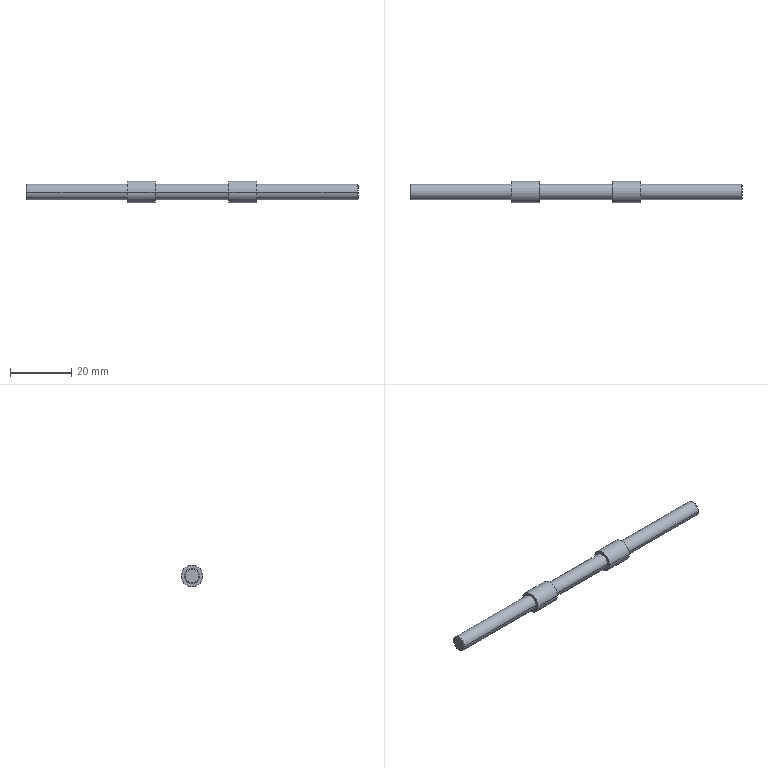Part | SolidWorks | features BaseBody 1 | 1 solid | 20 faces | box 108 x 7 x 7 mm | volume 2459 mm3 | cylinder 10 | plane 6 | cone 4 | commonest cylinder face diameters 5 x6 7 x4
STEP:
#1=CARTESIAN_POINT('',(0.,-2.25,0.));
#2=VERTEX_POINT('',#1);
#3=CARTESIAN_POINT('',(0.,2.25,0.));
#4=VERTEX_POINT('',#3);
#5=CARTESIAN_POINT('',(0.,0.,0.));
#6=DIRECTION('',(1.,0.,0.));
#7=DIRECTION('',(0.,-1.,0.));
#8=AXIS2_PLACEMENT_3D('',#5,#6,#7);
#9=CIRCLE('',#8,2.25);
#10=EDGE_CURVE('',#2,#4,#9,.T.);
#11=ORIENTED_EDGE('',*,*,#10,.T.);
#12=CARTESIAN_POINT('',(0.25,2.5,0.));
#13=VERTEX_POINT('',#12);
#14=CARTESIAN_POINT('',(0.125,2.375,0.));
#15=DIRECTION('',(0.7071,0.7071,0.));
#16=VECTOR('',#15,1000.);
#17=LINE('',#14,#16);
#18=EDGE_CURVE('',#4,#13,#17,.T.);
#19=ORIENTED_EDGE('',*,*,#18,.T.);
#20=CARTESIAN_POINT('',(0.25,-2.5,0.));
#21=VERTEX_POINT('',#20);
#22=CARTESIAN_POINT('',(0.25,0.,0.));
#23=DIRECTION('',(-1.,0.,0.));
#24=DIRECTION('',(0.,-1.,0.));
#25=AXIS2_PLACEMENT_3D('',#22,#23,#24);
#26=CIRCLE('',#25,2.5);
#27=EDGE_CURVE('',#13,#21,#26,.T.);
#28=ORIENTED_EDGE('',*,*,#27,.T.);
#29=CARTESIAN_POINT('',(0.125,-2.375,0.));
#30=DIRECTION('',(0.7071,-0.7071,0.));
#31=VECTOR('',#30,1000.);
#32=LINE('',#29,#31);
#33=EDGE_CURVE('',#2,#21,#32,.T.);
#34=ORIENTED_EDGE('',*,*,#33,.F.);
#35=EDGE_LOOP('',(#11,#19,#28,#34));
#36=FACE_OUTER_BOUND('',#35,.T.);
#37=CARTESIAN_POINT('',(0.125,0.,0.));
#38=DIRECTION('',(1.,0.,0.));
#39=DIRECTION('',(0.,-1.,0.));
#40=AXIS2_PLACEMENT_3D('',#37,#38,#39);
#41=CONICAL_SURFACE('',#40,2.375,0.7854);
#42=ADVANCED_FACE('',(#36),#41,.T.);
#43=CARTESIAN_POINT('',(33.,-2.5,0.));
#44=VERTEX_POINT('',#43);
#45=CARTESIAN_POINT('',(33.,2.5,0.));
#46=VERTEX_POINT('',#45);
#47=CARTESIAN_POINT('',(33.,0.,0.));
#48=DIRECTION('',(1.,0.,0.));
#49=DIRECTION('',(0.,0.,-1.));
#50=AXIS2_PLACEMENT_3D('',#47,#48,#49);
#51=CIRCLE('',#50,2.5);
#52=EDGE_CURVE('',#44,#46,#51,.T.);
#53=ORIENTED_EDGE('',*,*,#52,.F.);
#54=CARTESIAN_POINT('',(19.,-2.5,0.));
#55=DIRECTION('',(-1.,0.,0.));
#56=VECTOR('',#55,1000.);
#57=LINE('',#54,#56);
#58=EDGE_CURVE('',#44,#21,#57,.T.);
#59=ORIENTED_EDGE('',*,*,#58,.T.);
#60=ORIENTED_EDGE('',*,*,#27,.F.);
#61=CARTESIAN_POINT('',(19.,2.5,0.));
#62=DIRECTION('',(-1.,0.,0.));
#63=VECTOR('',#62,1000.);
#64=LINE('',#61,#63);
#65=EDGE_CURVE('',#46,#13,#64,.T.);
#66=ORIENTED_EDGE('',*,*,#65,.F.);
#67=EDGE_LOOP('',(#53,#59,#60,#66));
#68=FACE_OUTER_BOUND('',#67,.T.);
#69=CARTESIAN_POINT('',(19.,0.,0.));
#70=DIRECTION('',(-1.,0.,0.));
#71=DIRECTION('',(0.,1.,0.));
#72=AXIS2_PLACEMENT_3D('',#69,#70,#71);
#73=CYLINDRICAL_SURFACE('',#72,2.5);
#74=ADVANCED_FACE('',(#68),#73,.T.);
#75=CARTESIAN_POINT('',(108.,-2.25,0.));
#76=VERTEX_POINT('',#75);
#77=CARTESIAN_POINT('',(108.,2.25,0.));
#78=VERTEX_POINT('',#77);
#79=CARTESIAN_POINT('',(108.,0.,0.));
#80=DIRECTION('',(-1.,0.,0.));
#81=DIRECTION('',(0.,-1.,0.));
#82=AXIS2_PLACEMENT_3D('',#79,#80,#81);
#83=CIRCLE('',#82,2.25);
#84=EDGE_CURVE('',#76,#78,#83,.T.);
#85=ORIENTED_EDGE('',*,*,#84,.T.);
#86=CARTESIAN_POINT('',(107.75,2.5,0.));
#87=VERTEX_POINT('',#86);
#88=CARTESIAN_POINT('',(107.875,2.375,0.));
#89=DIRECTION('',(-0.7071,0.7071,0.));
#90=VECTOR('',#89,1000.);
#91=LINE('',#88,#90);
#92=EDGE_CURVE('',#78,#87,#91,.T.);
#93=ORIENTED_EDGE('',*,*,#92,.T.);
#94=CARTESIAN_POINT('',(107.75,-2.5,0.));
#95=VERTEX_POINT('',#94);
#96=CARTESIAN_POINT('',(107.75,0.,0.));
#97=DIRECTION('',(1.,0.,0.));
#98=DIRECTION('',(0.,-1.,0.));
#99=AXIS2_PLACEMENT_3D('',#96,#97,#98);
#100=CIRCLE('',#99,2.5);
#101=EDGE_CURVE('',#87,#95,#100,.T.);
#102=ORIENTED_EDGE('',*,*,#101,.T.);
#103=CARTESIAN_POINT('',(107.875,-2.375,0.));
#104=DIRECTION('',(-0.7071,-0.7071,0.));
#105=VECTOR('',#104,1000.);
#106=LINE('',#103,#105);
#107=EDGE_CURVE('',#76,#95,#106,.T.);
#108=ORIENTED_EDGE('',*,*,#107,.F.);
#109=EDGE_LOOP('',(#85,#93,#102,#108));
#110=FACE_OUTER_BOUND('',#109,.T.);
#111=CARTESIAN_POINT('',(107.875,0.,0.));
#112=DIRECTION('',(-1.,0.,0.));
#113=DIRECTION('',(0.,-1.,0.));
#114=AXIS2_PLACEMENT_3D('',#111,#112,#113);
#115=CONICAL_SURFACE('',#114,2.375,0.7854);
#116=ADVANCED_FACE('',(#110),#115,.T.);
#117=CARTESIAN_POINT('',(107.75,0.,0.));
#118=DIRECTION('',(1.,0.,0.));
#119=DIRECTION('',(0.,-1.,0.));
#120=AXIS2_PLACEMENT_3D('',#117,#118,#119);
#121=CIRCLE('',#120,2.5);
#122=EDGE_CURVE('',#95,#87,#121,.T.);
#123=ORIENTED_EDGE('',*,*,#122,.F.);
#124=CARTESIAN_POINT('',(75.,-2.5,0.));
#125=VERTEX_POINT('',#124);
#126=CARTESIAN_POINT('',(91.5,-2.5,0.));
#127=DIRECTION('',(-1.,0.,0.));
#128=VECTOR('',#127,1000.);
#129=LINE('',#126,#128);
#130=EDGE_CURVE('',#95,#125,#129,.T.);
#131=ORIENTED_EDGE('',*,*,#130,.T.);
#132=CARTESIAN_POINT('',(75.,2.5,0.));
#133=VERTEX_POINT('',#132);
#134=CARTESIAN_POINT('',(75.,0.,0.));
#135=DIRECTION('',(1.,0.,0.));
#136=DIRECTION('',(0.,0.,-1.));
#137=AXIS2_PLACEMENT_3D('',#134,#135,#136);
#138=CIRCLE('',#137,2.5);
#139=EDGE_CURVE('',#125,#133,#138,.T.);
#140=ORIENTED_EDGE('',*,*,#139,.T.);
#141=CARTESIAN_POINT('',(91.5,2.5,0.));
#142=DIRECTION('',(-1.,0.,0.));
#143=VECTOR('',#142,1000.);
#144=LINE('',#141,#143);
#145=EDGE_CURVE('',#87,#133,#144,.T.);
#146=ORIENTED_EDGE('',*,*,#145,.F.);
#147=EDGE_LOOP('',(#123,#131,#140,#146));
#148=FACE_OUTER_BOUND('',#147,.T.);
#149=CARTESIAN_POINT('',(91.5,0.,0.));
#150=DIRECTION('',(-1.,0.,0.));
#151=DIRECTION('',(0.,1.,0.));
#152=AXIS2_PLACEMENT_3D('',#149,#150,#151);
#153=CYLINDRICAL_SURFACE('',#152,2.5);
#154=ADVANCED_FACE('',(#148),#153,.T.);
#155=CARTESIAN_POINT('',(42.,-3.5,0.));
#156=VERTEX_POINT('',#155);
#157=CARTESIAN_POINT('',(42.,3.5,0.));
#158=VERTEX_POINT('',#157);
#159=CARTESIAN_POINT('',(42.,0.,0.));
#160=DIRECTION('',(1.,0.,0.));
#161=DIRECTION('',(0.,0.,-1.));
#162=AXIS2_PLACEMENT_3D('',#159,#160,#161);
#163=CIRCLE('',#162,3.5);
#164=EDGE_CURVE('',#156,#158,#163,.T.);
#165=ORIENTED_EDGE('',*,*,#164,.F.);
#166=CARTESIAN_POINT('',(33.,-3.5,0.));
#167=VERTEX_POINT('',#166);
#168=CARTESIAN_POINT('',(37.5,-3.5,0.));
#169=DIRECTION('',(-1.,0.,0.));
#170=VECTOR('',#169,1000.);
#171=LINE('',#168,#170);
#172=EDGE_CURVE('',#156,#167,#171,.T.);
#173=ORIENTED_EDGE('',*,*,#172,.T.);
#174=CARTESIAN_POINT('',(33.,3.5,0.));
#175=VERTEX_POINT('',#174);
#176=CARTESIAN_POINT('',(33.,0.,0.));
#177=DIRECTION('',(1.,0.,0.));
#178=DIRECTION('',(0.,0.,-1.));
#179=AXIS2_PLACEMENT_3D('',#176,#177,#178);
#180=CIRCLE('',#179,3.5);
#181=EDGE_CURVE('',#167,#175,#180,.T.);
#182=ORIENTED_EDGE('',*,*,#181,.T.);
#183=CARTESIAN_POINT('',(37.5,3.5,0.));
#184=DIRECTION('',(-1.,0.,0.));
#185=VECTOR('',#184,1000.);
#186=LINE('',#183,#185);
#187=EDGE_CURVE('',#158,#175,#186,.T.);
#188=ORIENTED_EDGE('',*,*,#187,.F.);
#189=EDGE_LOOP('',(#165,#173,#182,#188));
#190=FACE_OUTER_BOUND('',#189,.T.);
#191=CARTESIAN_POINT('',(37.5,0.,0.));
#192=DIRECTION('',(-1.,0.,0.));
#193=DIRECTION('',(0.,1.,0.));
#194=AXIS2_PLACEMENT_3D('',#191,#192,#193);
#195=CYLINDRICAL_SURFACE('',#194,3.5);
#196=ADVANCED_FACE('',(#190),#195,.T.);
#197=CARTESIAN_POINT('',(66.,-2.5,0.));
#198=VERTEX_POINT('',#197);
#199=CARTESIAN_POINT('',(66.,2.5,0.));
#200=VERTEX_POINT('',#199);
#201=CARTESIAN_POINT('',(66.,0.,0.));
#202=DIRECTION('',(1.,0.,0.));
#203=DIRECTION('',(0.,0.,-1.));
#204=AXIS2_PLACEMENT_3D('',#201,#202,#203);
#205=CIRCLE('',#204,2.5);
#206=EDGE_CURVE('',#198,#200,#205,.T.);
#207=ORIENTED_EDGE('',*,*,#206,.F.);
#208=CARTESIAN_POINT('',(42.,-2.5,0.));
#209=VERTEX_POINT('',#208);
#210=CARTESIAN_POINT('',(54.,-2.5,0.));
#211=DIRECTION('',(-1.,0.,0.));
#212=VECTOR('',#211,1000.);
#213=LINE('',#210,#212);
#214=EDGE_CURVE('',#198,#209,#213,.T.);
#215=ORIENTED_EDGE('',*,*,#214,.T.);
#216=CARTESIAN_POINT('',(42.,2.5,0.));
#217=VERTEX_POINT('',#216);
#218=CARTESIAN_POINT('',(42.,0.,0.));
#219=DIRECTION('',(1.,0.,0.));
#220=DIRECTION('',(0.,0.,-1.));
#221=AXIS2_PLACEMENT_3D('',#218,#219,#220);
#222=CIRCLE('',#221,2.5);
#223=EDGE_CURVE('',#209,#217,#222,.T.);
#224=ORIENTED_EDGE('',*,*,#223,.T.);
#225=CARTESIAN_POINT('',(54.,2.5,0.));
#226=DIRECTION('',(-1.,0.,0.));
#227=VECTOR('',#226,1000.);
#228=LINE('',#225,#227);
#229=EDGE_CURVE('',#200,#217,#228,.T.);
#230=ORIENTED_EDGE('',*,*,#229,.F.);
#231=EDGE_LOOP('',(#207,#215,#224,#230));
#232=FACE_OUTER_BOUND('',#231,.T.);
#233=CARTESIAN_POINT('',(54.,0.,0.));
#234=DIRECTION('',(-1.,0.,0.));
#235=DIRECTION('',(0.,1.,0.));
#236=AXIS2_PLACEMENT_3D('',#233,#234,#235);
#237=CYLINDRICAL_SURFACE('',#236,2.5);
#238=ADVANCED_FACE('',(#232),#237,.T.);
#239=CARTESIAN_POINT('',(75.,-3.5,0.));
#240=VERTEX_POINT('',#239);
#241=CARTESIAN_POINT('',(75.,3.5,0.));
#242=VERTEX_POINT('',#241);
#243=CARTESIAN_POINT('',(75.,0.,0.));
#244=DIRECTION('',(1.,0.,0.));
#245=DIRECTION('',(0.,0.,-1.));
#246=AXIS2_PLACEMENT_3D('',#243,#244,#245);
#247=CIRCLE('',#246,3.5);
#248=EDGE_CURVE('',#240,#242,#247,.T.);
#249=ORIENTED_EDGE('',*,*,#248,.F.);
#250=CARTESIAN_POINT('',(66.,-3.5,0.));
#251=VERTEX_POINT('',#250);
#252=CARTESIAN_POINT('',(70.5,-3.5,0.));
#253=DIRECTION('',(-1.,0.,0.));
#254=VECTOR('',#253,1000.);
#255=LINE('',#252,#254);
#256=EDGE_CURVE('',#240,#251,#255,.T.);
#257=ORIENTED_EDGE('',*,*,#256,.T.);
#258=CARTESIAN_POINT('',(66.,3.5,0.));
#259=VERTEX_POINT('',#258);
#260=CARTESIAN_POINT('',(66.,0.,0.));
#261=DIRECTION('',(1.,0.,0.));
#262=DIRECTION('',(0.,0.,-1.));
#263=AXIS2_PLACEMENT_3D('',#260,#261,#262);
#264=CIRCLE('',#263,3.5);
#265=EDGE_CURVE('',#251,#259,#264,.T.);
#266=ORIENTED_EDGE('',*,*,#265,.T.);
#267=CARTESIAN_POINT('',(70.5,3.5,0.));
#268=DIRECTION('',(-1.,0.,0.));
#269=VECTOR('',#268,1000.);
#270=LINE('',#267,#269);
#271=EDGE_CURVE('',#242,#259,#270,.T.);
#272=ORIENTED_EDGE('',*,*,#271,.F.);
#273=EDGE_LOOP('',(#249,#257,#266,#272));
#274=FACE_OUTER_BOUND('',#273,.T.);
#275=CARTESIAN_POINT('',(70.5,0.,0.));
#276=DIRECTION('',(-1.,0.,0.));
#277=DIRECTION('',(0.,1.,0.));
#278=AXIS2_PLACEMENT_3D('',#275,#276,#277);
#279=CYLINDRICAL_SURFACE('',#278,3.5);
#280=ADVANCED_FACE('',(#274),#279,.T.);
#281=ORIENTED_EDGE('',*,*,#10,.F.);
#282=CARTESIAN_POINT('',(0.,0.,0.));
#283=DIRECTION('',(1.,0.,0.));
#284=DIRECTION('',(0.,-1.,0.));
#285=AXIS2_PLACEMENT_3D('',#282,#283,#284);
#286=CIRCLE('',#285,2.25);
#287=EDGE_CURVE('',#4,#2,#286,.T.);
#288=ORIENTED_EDGE('',*,*,#287,.F.);
#289=EDGE_LOOP('',(#281,#288));
#290=FACE_OUTER_BOUND('',#289,.T.);
#291=CARTESIAN_POINT('',(0.,2.5,0.));
#292=DIRECTION('',(-1.,0.,0.));
#293=DIRECTION('',(0.,0.,1.));
#294=AXIS2_PLACEMENT_3D('',#291,#292,#293);
#295=PLANE('',#294);
#296=ADVANCED_FACE('',(#290),#295,.T.);
#297=ORIENTED_EDGE('',*,*,#84,.F.);
#298=CARTESIAN_POINT('',(108.,0.,0.));
#299=DIRECTION('',(-1.,0.,0.));
#300=DIRECTION('',(0.,-1.,0.));
#301=AXIS2_PLACEMENT_3D('',#298,#299,#300);
#302=CIRCLE('',#301,2.25);
#303=EDGE_CURVE('',#78,#76,#302,.T.);
#304=ORIENTED_EDGE('',*,*,#303,.F.);
#305=EDGE_LOOP('',(#297,#304));
#306=FACE_OUTER_BOUND('',#305,.T.);
#307=CARTESIAN_POINT('',(108.,0.,0.));
#308=DIRECTION('',(1.,0.,0.));
#309=DIRECTION('',(0.,1.,0.));
#310=AXIS2_PLACEMENT_3D('',#307,#308,#309);
#311=PLANE('',#310);
#312=ADVANCED_FACE('',(#306),#311,.T.);
#313=CARTESIAN_POINT('',(33.,0.,0.));
#314=DIRECTION('',(1.,0.,0.));
#315=DIRECTION('',(0.,0.,-1.));
#316=AXIS2_PLACEMENT_3D('',#313,#314,#315);
#317=CIRCLE('',#316,2.5);
#318=EDGE_CURVE('',#46,#44,#317,.T.);
#319=ORIENTED_EDGE('',*,*,#318,.T.);
#320=ORIENTED_EDGE('',*,*,#52,.T.);
#321=EDGE_LOOP('',(#319,#320));
#322=FACE_BOUND('',#321,.T.);
#323=CARTESIAN_POINT('',(33.,0.,0.));
#324=DIRECTION('',(1.,0.,0.));
#325=DIRECTION('',(0.,0.,-1.));
#326=AXIS2_PLACEMENT_3D('',#323,#324,#325);
#327=CIRCLE('',#326,3.5);
#328=EDGE_CURVE('',#175,#167,#327,.T.);
#329=ORIENTED_EDGE('',*,*,#328,.F.);
#330=ORIENTED_EDGE('',*,*,#181,.F.);
#331=EDGE_LOOP('',(#329,#330));
#332=FACE_OUTER_BOUND('',#331,.T.);
#333=CARTESIAN_POINT('',(33.,3.5,0.));
#334=DIRECTION('',(-1.,0.,0.));
#335=DIRECTION('',(0.,0.,1.));
#336=AXIS2_PLACEMENT_3D('',#333,#334,#335);
#337=PLANE('',#336);
#338=ADVANCED_FACE('',(#322,#332),#337,.T.);
#339=CARTESIAN_POINT('',(42.,0.,0.));
#340=DIRECTION('',(1.,0.,0.));
#341=DIRECTION('',(0.,0.,-1.));
#342=AXIS2_PLACEMENT_3D('',#339,#340,#341);
#343=CIRCLE('',#342,2.5);
#344=EDGE_CURVE('',#217,#209,#343,.T.);
#345=ORIENTED_EDGE('',*,*,#344,.F.);
#346=ORIENTED_EDGE('',*,*,#223,.F.);
#347=EDGE_LOOP('',(#345,#346));
#348=FACE_BOUND('',#347,.T.);
#349=CARTESIAN_POINT('',(42.,0.,0.));
#350=DIRECTION('',(1.,0.,0.));
#351=DIRECTION('',(0.,0.,-1.));
#352=AXIS2_PLACEMENT_3D('',#349,#350,#351);
#353=CIRCLE('',#352,3.5);
#354=EDGE_CURVE('',#158,#156,#353,.T.);
#355=ORIENTED_EDGE('',*,*,#354,.T.);
#356=ORIENTED_EDGE('',*,*,#164,.T.);
#357=EDGE_LOOP('',(#355,#356));
#358=FACE_OUTER_BOUND('',#357,.T.);
#359=CARTESIAN_POINT('',(42.,2.5,0.));
#360=DIRECTION('',(1.,0.,0.));
#361=DIRECTION('',(0.,1.,0.));
#362=AXIS2_PLACEMENT_3D('',#359,#360,#361);
#363=PLANE('',#362);
#364=ADVANCED_FACE('',(#348,#358),#363,.T.);
#365=CARTESIAN_POINT('',(66.,0.,0.));
#366=DIRECTION('',(1.,0.,0.));
#367=DIRECTION('',(0.,0.,-1.));
#368=AXIS2_PLACEMENT_3D('',#365,#366,#367);
#369=CIRCLE('',#368,2.5);
#370=EDGE_CURVE('',#200,#198,#369,.T.);
#371=ORIENTED_EDGE('',*,*,#370,.T.);
#372=ORIENTED_EDGE('',*,*,#206,.T.);
#373=EDGE_LOOP('',(#371,#372));
#374=FACE_BOUND('',#373,.T.);
#375=CARTESIAN_POINT('',(66.,0.,0.));
#376=DIRECTION('',(1.,0.,0.));
#377=DIRECTION('',(0.,0.,-1.));
#378=AXIS2_PLACEMENT_3D('',#375,#376,#377);
#379=CIRCLE('',#378,3.5);
#380=EDGE_CURVE('',#259,#251,#379,.T.);
#381=ORIENTED_EDGE('',*,*,#380,.F.);
#382=ORIENTED_EDGE('',*,*,#265,.F.);
#383=EDGE_LOOP('',(#381,#382));
#384=FACE_OUTER_BOUND('',#383,.T.);
#385=CARTESIAN_POINT('',(66.,3.5,0.));
#386=DIRECTION('',(-1.,0.,0.));
#387=DIRECTION('',(0.,0.,1.));
#388=AXIS2_PLACEMENT_3D('',#385,#386,#387);
#389=PLANE('',#388);
#390=ADVANCED_FACE('',(#374,#384),#389,.T.);
#391=CARTESIAN_POINT('',(75.,0.,0.));
#392=DIRECTION('',(1.,0.,0.));
#393=DIRECTION('',(0.,0.,-1.));
#394=AXIS2_PLACEMENT_3D('',#391,#392,#393);
#395=CIRCLE('',#394,2.5);
#396=EDGE_CURVE('',#133,#125,#395,.T.);
#397=ORIENTED_EDGE('',*,*,#396,.F.);
#398=ORIENTED_EDGE('',*,*,#139,.F.);
#399=EDGE_LOOP('',(#397,#398));
#400=FACE_BOUND('',#399,.T.);
#401=CARTESIAN_POINT('',(75.,0.,0.));
#402=DIRECTION('',(1.,0.,0.));
#403=DIRECTION('',(0.,0.,-1.));
#404=AXIS2_PLACEMENT_3D('',#401,#402,#403);
#405=CIRCLE('',#404,3.5);
#406=EDGE_CURVE('',#242,#240,#405,.T.);
#407=ORIENTED_EDGE('',*,*,#406,.T.);
#408=ORIENTED_EDGE('',*,*,#248,.T.);
#409=EDGE_LOOP('',(#407,#408));
#410=FACE_OUTER_BOUND('',#409,.T.);
#411=CARTESIAN_POINT('',(75.,2.5,0.));
#412=DIRECTION('',(1.,0.,0.));
#413=DIRECTION('',(0.,1.,0.));
#414=AXIS2_PLACEMENT_3D('',#411,#412,#413);
#415=PLANE('',#414);
#416=ADVANCED_FACE('',(#400,#410),#415,.T.);
#417=ORIENTED_EDGE('',*,*,#256,.F.);
#418=ORIENTED_EDGE('',*,*,#406,.F.);
#419=ORIENTED_EDGE('',*,*,#271,.T.);
#420=ORIENTED_EDGE('',*,*,#380,.T.);
#421=EDGE_LOOP('',(#417,#418,#419,#420));
#422=FACE_OUTER_BOUND('',#421,.T.);
#423=CARTESIAN_POINT('',(70.5,0.,0.));
#424=DIRECTION('',(-1.,0.,0.));
#425=DIRECTION('',(0.,1.,0.));
#426=AXIS2_PLACEMENT_3D('',#423,#424,#425);
#427=CYLINDRICAL_SURFACE('',#426,3.5);
#428=ADVANCED_FACE('',(#422),#427,.T.);
#429=ORIENTED_EDGE('',*,*,#214,.F.);
#430=ORIENTED_EDGE('',*,*,#370,.F.);
#431=ORIENTED_EDGE('',*,*,#229,.T.);
#432=ORIENTED_EDGE('',*,*,#344,.T.);
#433=EDGE_LOOP('',(#429,#430,#431,#432));
#434=FACE_OUTER_BOUND('',#433,.T.);
#435=CARTESIAN_POINT('',(54.,0.,0.));
#436=DIRECTION('',(-1.,0.,0.));
#437=DIRECTION('',(0.,1.,0.));
#438=AXIS2_PLACEMENT_3D('',#435,#436,#437);
#439=CYLINDRICAL_SURFACE('',#438,2.5);
#440=ADVANCED_FACE('',(#434),#439,.T.);
#441=ORIENTED_EDGE('',*,*,#172,.F.);
#442=ORIENTED_EDGE('',*,*,#354,.F.);
#443=ORIENTED_EDGE('',*,*,#187,.T.);
#444=ORIENTED_EDGE('',*,*,#328,.T.);
#445=EDGE_LOOP('',(#441,#442,#443,#444));
#446=FACE_OUTER_BOUND('',#445,.T.);
#447=CARTESIAN_POINT('',(37.5,0.,0.));
#448=DIRECTION('',(-1.,0.,0.));
#449=DIRECTION('',(0.,1.,0.));
#450=AXIS2_PLACEMENT_3D('',#447,#448,#449);
#451=CYLINDRICAL_SURFACE('',#450,3.5);
#452=ADVANCED_FACE('',(#446),#451,.T.);
#453=ORIENTED_EDGE('',*,*,#130,.F.);
#454=ORIENTED_EDGE('',*,*,#101,.F.);
#455=ORIENTED_EDGE('',*,*,#145,.T.);
#456=ORIENTED_EDGE('',*,*,#396,.T.);
#457=EDGE_LOOP('',(#453,#454,#455,#456));
#458=FACE_OUTER_BOUND('',#457,.T.);
#459=CARTESIAN_POINT('',(91.5,0.,0.));
#460=DIRECTION('',(-1.,0.,0.));
#461=DIRECTION('',(0.,1.,0.));
#462=AXIS2_PLACEMENT_3D('',#459,#460,#461);
#463=CYLINDRICAL_SURFACE('',#462,2.5);
#464=ADVANCED_FACE('',(#458),#463,.T.);
#465=ORIENTED_EDGE('',*,*,#92,.F.);
#466=ORIENTED_EDGE('',*,*,#303,.T.);
#467=ORIENTED_EDGE('',*,*,#107,.T.);
#468=ORIENTED_EDGE('',*,*,#122,.T.);
#469=EDGE_LOOP('',(#465,#466,#467,#468));
#470=FACE_OUTER_BOUND('',#469,.T.);
#471=CARTESIAN_POINT('',(107.875,0.,0.));
#472=DIRECTION('',(-1.,0.,0.));
#473=DIRECTION('',(0.,-1.,0.));
#474=AXIS2_PLACEMENT_3D('',#471,#472,#473);
#475=CONICAL_SURFACE('',#474,2.375,0.7854);
#476=ADVANCED_FACE('',(#470),#475,.T.);
#477=ORIENTED_EDGE('',*,*,#58,.F.);
#478=ORIENTED_EDGE('',*,*,#318,.F.);
#479=ORIENTED_EDGE('',*,*,#65,.T.);
#480=CARTESIAN_POINT('',(0.25,0.,0.));
#481=DIRECTION('',(-1.,0.,0.));
#482=DIRECTION('',(0.,-1.,0.));
#483=AXIS2_PLACEMENT_3D('',#480,#481,#482);
#484=CIRCLE('',#483,2.5);
#485=EDGE_CURVE('',#21,#13,#484,.T.);
#486=ORIENTED_EDGE('',*,*,#485,.F.);
#487=EDGE_LOOP('',(#477,#478,#479,#486));
#488=FACE_OUTER_BOUND('',#487,.T.);
#489=CARTESIAN_POINT('',(19.,0.,0.));
#490=DIRECTION('',(-1.,0.,0.));
#491=DIRECTION('',(0.,1.,0.));
#492=AXIS2_PLACEMENT_3D('',#489,#490,#491);
#493=CYLINDRICAL_SURFACE('',#492,2.5);
#494=ADVANCED_FACE('',(#488),#493,.T.);
#495=ORIENTED_EDGE('',*,*,#18,.F.);
#496=ORIENTED_EDGE('',*,*,#287,.T.);
#497=ORIENTED_EDGE('',*,*,#33,.T.);
#498=ORIENTED_EDGE('',*,*,#485,.T.);
#499=EDGE_LOOP('',(#495,#496,#497,#498));
#500=FACE_OUTER_BOUND('',#499,.T.);
#501=CARTESIAN_POINT('',(0.125,0.,0.));
#502=DIRECTION('',(1.,0.,0.));
#503=DIRECTION('',(0.,-1.,0.));
#504=AXIS2_PLACEMENT_3D('',#501,#502,#503);
#505=CONICAL_SURFACE('',#504,2.375,0.7854);
#506=ADVANCED_FACE('',(#500),#505,.T.);
#507=CLOSED_SHELL('',(#42,#74,#116,#154,#196,#238,#280,#296,#312,#338,#364,#390,#416,#428,#440,#452,#464,#476,#494,#506));
#508=MANIFOLD_SOLID_BREP('',#507);
#509=CARTESIAN_POINT('',(0.,0.,0.));
#510=DIRECTION('',(0.,0.,1.));
#511=DIRECTION('',(1.,0.,0.));
#512=AXIS2_PLACEMENT_3D('',#509,#510,#511);
#513=(LENGTH_UNIT()NAMED_UNIT(*)SI_UNIT(.MILLI.,.METRE.));
#514=UNCERTAINTY_MEASURE_WITH_UNIT(LENGTH_MEASURE(0.00001),#513,'','');
#515=(NAMED_UNIT(*)PLANE_ANGLE_UNIT()SI_UNIT($,.RADIAN.));
#516=(NAMED_UNIT(*)SI_UNIT($,.STERADIAN.)SOLID_ANGLE_UNIT());
#517=(GEOMETRIC_REPRESENTATION_CONTEXT(3)GLOBAL_UNCERTAINTY_ASSIGNED_CONTEXT((#514))GLOBAL_UNIT_ASSIGNED_CONTEXT((#513,#515,#516))REPRESENTATION_CONTEXT('',''));
#518=ADVANCED_BREP_SHAPE_REPRESENTATION('',(#508,#512),#517);